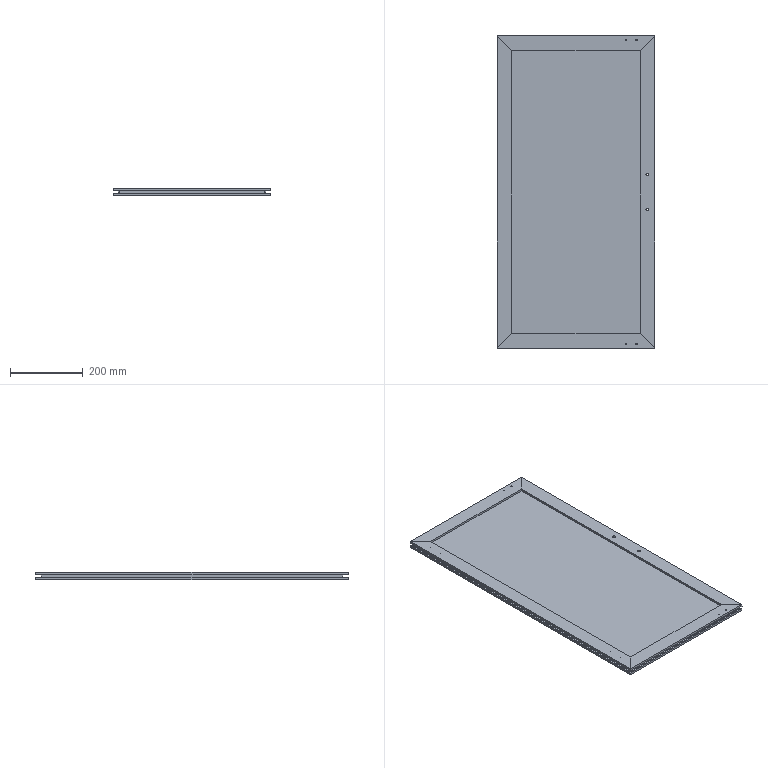Part | SolidWorks | features HoleWzd 3, ICE 1, WeldMemberFeat 1, WeldmentFeature 1 | 5 solids | 184 faces | box 432 x 856 x 20 mm | volume 2324012 mm3 | plane 132 | cylinder 44 | cone 8 | commonest cylinder face diameters 5 x16 3.3 x8 4.5 x8 6.5 x8 8 x4